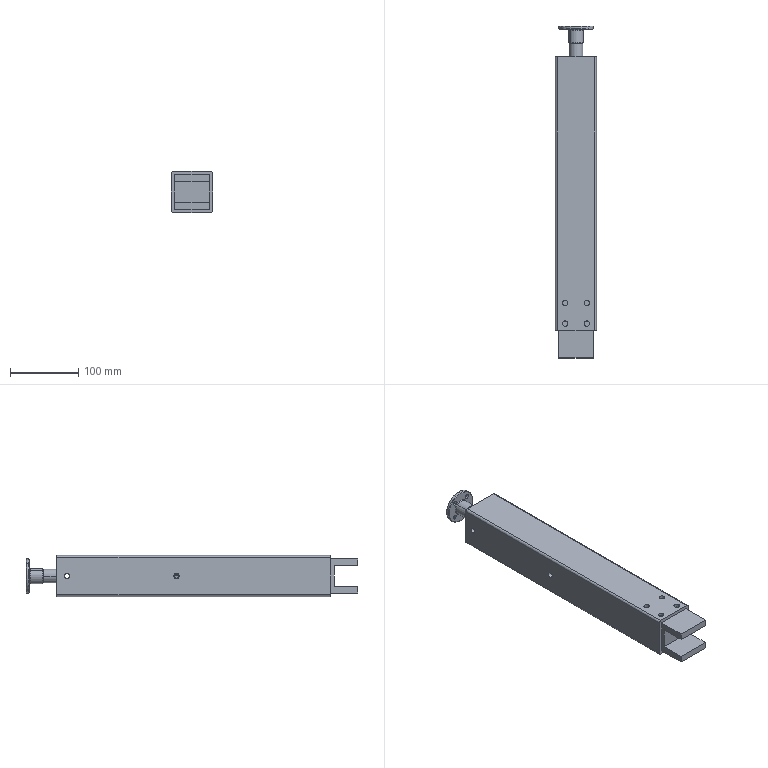Part | SolidWorks | 20 solids | 467 faces | box 60 x 485 x 60 mm | volume 1102301 mm3 | plane 240 | cylinder 178 | cone 40 | spline 5 | torus 4 | commonest cylinder face diameters 8 x46 32 x40 6 x24 5 x16 48 x14 20 x6